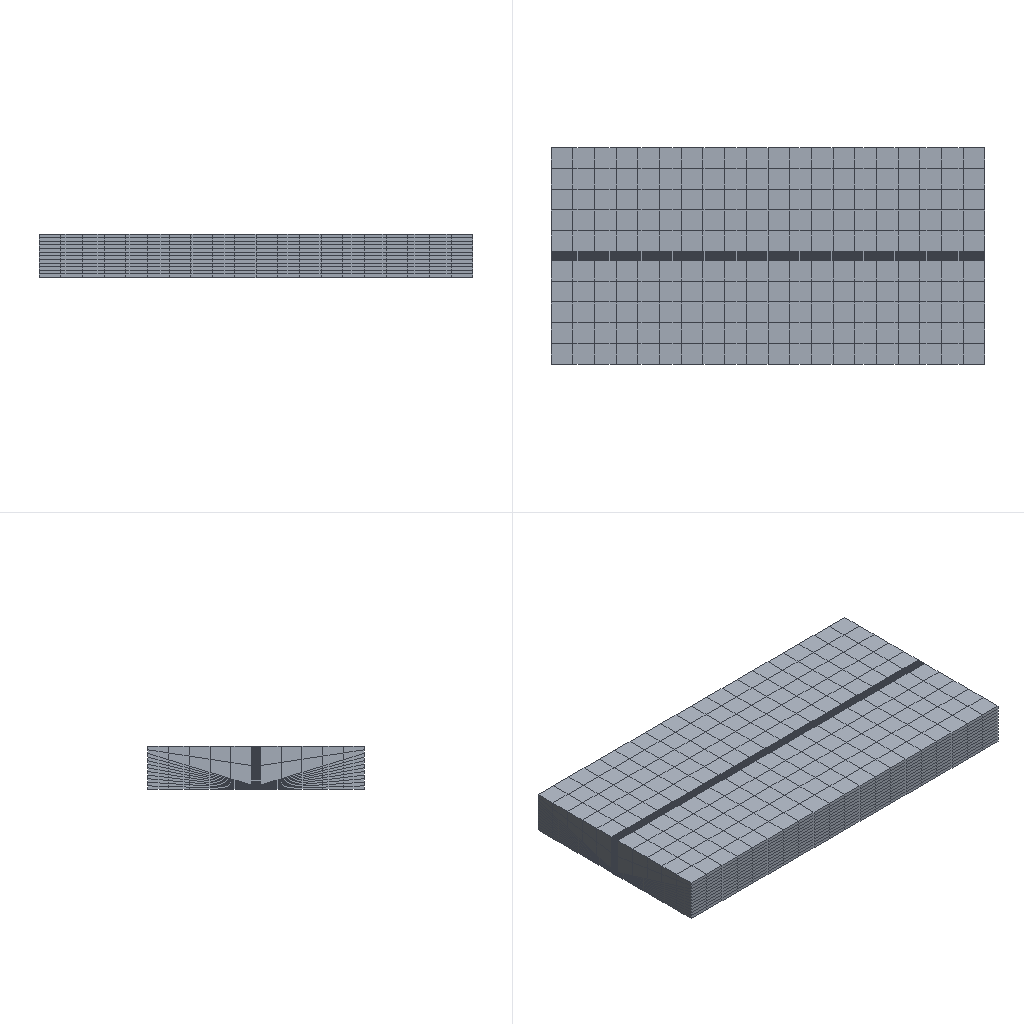Simulation study | abaqus
Set-up summary:
category,name,step,type,value,unit,region
solver,abaqus
solver,version,,,Abaqus/Standard 3DEXPERIENCE R2017x
units,not stated in the deck,,not stated
analysis,deck,,coupled temperature-displacement,coupled temperature-displacement
load_step,Step-1,Step-1,coupled temperature-displacement
load_step,requested,,,1
mesh,nodes,,,10685
mesh,elements,,,8200
element_type,C3D8RT,,solid,8200
load,load commands in deck,,count,3
bc,support commands in deck,,count,1
material,NI-TI,,in results
material,STEEL,,in results
check,setup vs results,,match,"per instance, exact: element labels, types and connectivity; labels of the nodes the elements use; coordinates of those nodes at SINGLE_PRECISION in 1 of 2 instance(s)"
Abaqus input file, long lists of numbers shortened:
*Heading
** Job name: 1011 Model name: Model-1
** Generated by: Abaqus/CAE 2017
*Preprint, echo=NO, model=NO, history=NO, contact=NO
**
** PARTS
**
*Part, name=Part-1
*Node
      1,           0.,         -24.,           0.
      2,           0.,         -26.,           0.
** (8461 more lines like these left out)
*Element, type=C3D8RT
   1,  212, 1201, 2821,  783,    1,   21,  403,   76
   2, 1201, 1202, 2822, 2821,   21,   22,  404,  403
** (7198 more lines like these left out)
*Nset, nset=Set-1, generate
    1,  8463,     1
*Elset, elset=Set-1, generate
    1,  7200,     1
** Section: STEEL
*Solid Section, elset=Set-1, material=STEEL
,
*End Part
**
*Part, name=Part-2
*Node
      1,         100.,          -1.,  0.1
      2,          99.,          -1.,  0.1
** (2220 more lines like these left out)
*Element, type=C3D8RT
   1,  203,  204,  305,  304,    1,    2,  103,  102
   2,  204,  205,  306,  305,    2,    3,  104,  103
** (998 more lines like these left out)
*Nset, nset=Set-1, generate
    1,  2222,     1
*Elset, elset=Set-1, generate
    1,  1000,     1
** Section: NI-TI
*Solid Section, elset=Set-1, material=NI-TI
,
*End Part
**
**
** ASSEMBLY
**
*Assembly, name=Assembly
**
*Instance, name=Part-1-1, part=Part-1
*End Instance
**
*Instance, name=Part-2-1, part=Part-2
          0.,        -24.5,         -0.1
*End Instance
**
*Node
      1,           0.,         -25., -0.1
*Node
      2,           0.,         -25., -0.1
*Nset, nset=Set-1, instance=Part-1-1
    1,    2,    3,    4,    7,   10,   13,   14,   15,   16,   17,   18,   19,   20,   21,   22
   23,   24,   25,   26,   27,   28,   29,   30,   31,   32,   33,   34,   35,   36,   37,   38
** (57 more lines like these left out)
*Nset, nset=Set-1, instance=Part-2-1, generate
    1,  2222,     1
*Elset, elset=Set-1, instance=Part-1-1
    1,    2,    3,    4,    5,    6,    7,    8,    9,   10,   11,   12,   13,   14,   15,   16
   17,   18,   19,   20,   21,   41,   61,   81,  101,  121,  141,  161,  181,  241,  242,  243
** (52 more lines like these left out)
*Elset, elset=Set-1, instance=Part-2-1, generate
    1,  1000,     1
*Nset, nset=Set-2, instance=Part-2-1, generate
    1,  2222,     1
*Elset, elset=Set-2, instance=Part-2-1, generate
    1,  1000,     1
*Nset, nset=Set-3, instance=Part-1-1
    1,    2,    7,   10,   18,   20,   21,   22,   23,   24,   25,   26,   27,   28,   29,   30
   31,   32,   33,   34,   35,   36,   37,   38,   39,   98,   99,  100,  101,  102,  103,  104
** (33 more lines like these left out)
*Elset, elset=Set-3, instance=Part-1-1
    1,    2,    3,    4,    5,    6,    7,    8,    9,   10,   11,   12,   13,   14,   15,   16
   17,   18,   19,   20,  241,  242,  243,  244,  245,  246,  247,  248,  249,  250,  251,  252
** (30 more lines like these left out)
*Nset, nset=Set-4, instance=Part-1-1, generate
    1,  8463,     1
*Nset, nset=Set-4, instance=Part-2-1, generate
    1,  2222,     1
*Elset, elset=Set-4, instance=Part-1-1, generate
    1,  7200,     1
*Elset, elset=Set-4, instance=Part-2-1, generate
    1,  1000,     1
*Nset, nset=Set-5, instance=Part-1-1
    5,    6,   11,   12,   14,   16,   17,   19,   78,   79,   80,   81,   82,   83,   84,   85
   86,   87,   88,   89,   90,   91,   92,   93,   94,   95,   96,  156,  157,  158,  159,  160
** (39 more lines like these left out)
*Elset, elset=Set-5, instance=Part-1-1
  221,  222,  223,  224,  225,  226,  227,  228,  229,  230,  231,  232,  233,  234,  235,  236
  237,  238,  239,  240,  461,  462,  463,  464,  465,  466,  467,  468,  469,  470,  471,  472
** (36 more lines like these left out)
*Nset, nset=Set-6, instance=Part-1-1, generate
    1,  8463,     1
*Nset, nset=Set-6, instance=Part-2-1, generate
    1,  2222,     1
*Elset, elset=Set-6, instance=Part-1-1, generate
    1,  7200,     1
*Elset, elset=Set-6, instance=Part-2-1, generate
    1,  1000,     1
*Elset, elset=_Surf-1_S5, internal, instance=Part-1-1
 6056, 6057, 6058, 6059, 6060, 6116, 6117, 6118, 6119, 6120, 6176, 6177, 6178, 6179, 6180, 6236
 6237, 6238, 6239, 6240, 6296, 6297, 6298, 6299, 6300, 6356, 6357, 6358, 6359, 6360, 6416, 6417
** (5 more lines like these left out)
*Elset, elset=_Surf-1_S5, internal, instance=Part-2-1, generate
    1,  1000,     1
*Elset, elset=_Surf-1_S3, internal, instance=Part-1-1
    1,    2,    3,    4,    5,    6,    7,    8,    9,   10,   11,   12,   13,   14,   15,   16
   17,   18,   19,   20,  241,  242,  243,  244,  245,  246,  247,  248,  249,  250,  251,  252
** (23 more lines like these left out)
*Elset, elset=_Surf-1_S3, internal, instance=Part-2-1, generate
    1,  1000,     1
*Elset, elset=_Surf-1_S4, internal, instance=Part-1-1
 4812, 4824, 4836, 4848, 4860, 4872, 4884, 4896, 4908, 4920, 4932, 4944, 4956, 4968, 4980, 4992
 5004, 5016, 5028, 5040, 5052, 5064, 5076, 5088, 5100, 5112, 5124, 5136, 5148, 5160, 5172, 5184
** (20 more lines like these left out)
*Elset, elset=_Surf-1_S4, internal, instance=Part-2-1, generate
  100,  1000,   100
*Elset, elset=_Surf-1_S1, internal, instance=Part-2-1, generate
  901,  1000,     1
*Elset, elset=_Surf-1_S2, internal, instance=Part-2-1, generate
   1,  100,    1
*Surface, type=ELEMENT, name=Surf-1
_Surf-1_S5, S5
_Surf-1_S3, S3
_Surf-1_S4, S4
_Surf-1_S2, S2
_Surf-1_S1, S1
*Elset, elset=_Surf-2_S5, internal, instance=Part-1-1
 6056, 6057, 6058, 6059, 6060, 6116, 6117, 6118, 6119, 6120, 6176, 6177, 6178, 6179, 6180, 6236
 6237, 6238, 6239, 6240, 6296, 6297, 6298, 6299, 6300, 6356, 6357, 6358, 6359, 6360, 6416, 6417
** (5 more lines like these left out)
*Elset, elset=_Surf-2_S5, internal, instance=Part-2-1, generate
    1,  1000,     1
*Elset, elset=_Surf-2_S3, internal, instance=Part-1-1
    1,    2,    3,    4,    5,    6,    7,    8,    9,   10,   11,   12,   13,   14,   15,   16
   17,   18,   19,   20,  241,  242,  243,  244,  245,  246,  247,  248,  249,  250,  251,  252
** (23 more lines like these left out)
*Elset, elset=_Surf-2_S3, internal, instance=Part-2-1, generate
    1,  1000,     1
*Elset, elset=_Surf-2_S4, internal, instance=Part-1-1
 4812, 4824, 4836, 4848, 4860, 4872, 4884, 4896, 4908, 4920, 4932, 4944, 4956, 4968, 4980, 4992
 5004, 5016, 5028, 5040, 5052, 5064, 5076, 5088, 5100, 5112, 5124, 5136, 5148, 5160, 5172, 5184
** (20 more lines like these left out)
*Elset, elset=_Surf-2_S4, internal, instance=Part-2-1, generate
  100,  1000,   100
*Elset, elset=_Surf-2_S1, internal, instance=Part-2-1, generate
  901,  1000,     1
*Elset, elset=_Surf-2_S2, internal, instance=Part-2-1, generate
   1,  100,    1
*Surface, type=ELEMENT, name=Surf-2
_Surf-2_S5, S5
_Surf-2_S3, S3
_Surf-2_S4, S4
_Surf-2_S2, S2
_Surf-2_S1, S1
*Elset, elset=_Surf-3_S2, internal, instance=Part-1-1
    1,    2,    3,    4,    5,    6,    7,    8,    9,   10,   11,   12,   13,   14,   15,   16
   17,   18,   19,   20,   21,   22,   23,   24,   25,   26,   27,   28,   29,   30,   31,   32
** (21 more lines like these left out)
*Elset, elset=_Surf-3_S2, internal, instance=Part-2-1, generate
   1,  100,    1
*Elset, elset=_Surf-3_S5, internal, instance=Part-1-1
  221,  222,  223,  224,  225,  226,  227,  228,  229,  230,  231,  232,  233,  234,  235,  236
  237,  238,  239,  240,  461,  462,  463,  464,  465,  466,  467,  468,  469,  470,  471,  472
** (45 more lines like these left out)
*Elset, elset=_Surf-3_S5, internal, instance=Part-2-1, generate
    1,  1000,     1
*Elset, elset=_Surf-3_S1, internal, instance=Part-1-1
 4561, 4562, 4563, 4564, 4565, 4566, 4567, 4568, 4569, 4570, 4571, 4572, 4573, 4574, 4575, 4576
 4577, 4578, 4579, 4580, 4581, 4582, 4583, 4584, 4585, 4586, 4587, 4588, 4589, 4590, 4591, 4592
** (21 more lines like these left out)
*Elset, elset=_Surf-3_S1, internal, instance=Part-2-1, generate
  901,  1000,     1
*Elset, elset=_Surf-3_S6, internal, instance=Part-1-1, generate
 4801,  5989,    12
*Elset, elset=_Surf-3_S6, internal, instance=Part-2-1, generate
   1,  901,  100
*Elset, elset=_Surf-3_S3, internal, instance=Part-1-1
    1,    2,    3,    4,    5,    6,    7,    8,    9,   10,   11,   12,   13,   14,   15,   16
   17,   18,   19,   20,  241,  242,  243,  244,  245,  246,  247,  248,  249,  250,  251,  252
** (30 more lines like these left out)
*Elset, elset=_Surf-3_S3, internal, instance=Part-2-1, generate
    1,  1000,     1
*Elset, elset=_Surf-3_S4, internal, instance=Part-1-1
 4812, 4824, 4836, 4848, 4860, 4872, 4884, 4896, 4908, 4920, 4932, 4944, 4956, 4968, 4980, 4992
 5004, 5016, 5028, 5040, 5052, 5064, 5076, 5088, 5100, 5112, 5124, 5136, 5148, 5160, 5172, 5184
** (20 more lines like these left out)
*Elset, elset=_Surf-3_S4, internal, instance=Part-2-1, generate
  100,  1000,   100
*Surface, type=ELEMENT, name=Surf-3
_Surf-3_S2, S2
_Surf-3_S5, S5
_Surf-3_S6, S6
_Surf-3_S4, S4
_Surf-3_S1, S1
_Surf-3_S3, S3
*Elset, elset=_Surf-4_S2, internal, instance=Part-1-1
    1,    2,    3,    4,    5,    6,    7,    8,    9,   10,   11,   12,   13,   14,   15,   16
   17,   18,   19,   20,   21,   22,   23,   24,   25,   26,   27,   28,   29,   30,   31,   32
** (21 more lines like these left out)
*Elset, elset=_Surf-4_S2, internal, instance=Part-2-1, generate
   1,  100,    1
*Elset, elset=_Surf-4_S5, internal, instance=Part-1-1
  221,  222,  223,  224,  225,  226,  227,  228,  229,  230,  231,  232,  233,  234,  235,  236
  237,  238,  239,  240,  461,  462,  463,  464,  465,  466,  467,  468,  469,  470,  471,  472
** (45 more lines like these left out)
*Elset, elset=_Surf-4_S5, internal, instance=Part-2-1, generate
    1,  1000,     1
*Elset, elset=_Surf-4_S1, internal, instance=Part-1-1
 4561, 4562, 4563, 4564, 4565, 4566, 4567, 4568, 4569, 4570, 4571, 4572, 4573, 4574, 4575, 4576
 4577, 4578, 4579, 4580, 4581, 4582, 4583, 4584, 4585, 4586, 4587, 4588, 4589, 4590, 4591, 4592
** (21 more lines like these left out)
*Elset, elset=_Surf-4_S1, internal, instance=Part-2-1, generate
  901,  1000,     1
*Elset, elset=_Surf-4_S6, internal, instance=Part-1-1, generate
 4801,  5989,    12
*Elset, elset=_Surf-4_S6, internal, instance=Part-2-1, generate
   1,  901,  100
*Elset, elset=_Surf-4_S3, internal, instance=Part-1-1
    1,    2,    3,    4,    5,    6,    7,    8,    9,   10,   11,   12,   13,   14,   15,   16
   17,   18,   19,   20,  241,  242,  243,  244,  245,  246,  247,  248,  249,  250,  251,  252
** (30 more lines like these left out)
*Elset, elset=_Surf-4_S3, internal, instance=Part-2-1, generate
    1,  1000,     1
*Elset, elset=_Surf-4_S4, internal, instance=Part-1-1
 4812, 4824, 4836, 4848, 4860, 4872, 4884, 4896, 4908, 4920, 4932, 4944, 4956, 4968, 4980, 4992
 5004, 5016, 5028, 5040, 5052, 5064, 5076, 5088, 5100, 5112, 5124, 5136, 5148, 5160, 5172, 5184
** (20 more lines like these left out)
*Elset, elset=_Surf-4_S4, internal, instance=Part-2-1, generate
  100,  1000,   100
*Surface, type=ELEMENT, name=Surf-4
_Surf-4_S2, S2
_Surf-4_S5, S5
_Surf-4_S6, S6
_Surf-4_S4, S4
_Surf-4_S1, S1
_Surf-4_S3, S3
*Elset, elset=_shang_S3, internal, instance=Part-1-1
    1,    2,    3,    4,    5,    6,    7,    8,    9,   10,   11,   12,   13,   14,   15,   16
   17,   18,   19,   20,  241,  242,  243,  244,  245,  246,  247,  248,  249,  250,  251,  252
** (23 more lines like these left out)
*Surface, type=ELEMENT, name=shang
_shang_S3, S3
*Elset, elset=_xia_S3, internal, instance=Part-2-1, generate
    1,  1000,     1
*Surface, type=ELEMENT, name=xia
_xia_S3, S3
** Constraint: Constraint-1
*Tie, name=Constraint-1, adjust=yes
shang, xia
*End Assembly
**
** MATERIALS
**
*Material, name=NI-TI
*Conductivity
10.,
*Density
 6.45e-09,
*Elastic
28000., 0.3
*Plastic
70.,0.
*Specific Heat
 3.2e+08,
*Material, name=STEEL
*Conductivity
 16.3,
*Density
 7.93e-09,
*Elastic
199000., 0.28
*Plastic
200.,0.
*Specific Heat
 5e+08,
**
** PHYSICAL CONSTANTS
**
*Physical Constants, absolute zero=-273.13, stefan boltzmann=5.67e-08
**
** PREDEFINED FIELDS
**
** Name: Predefined Field-1   Type: Temperature
*Initial Conditions, type=TEMPERATURE
Set-6, 20.
** ----------------------------------------------------------------
**
** STEP: Step-1
**
*Step, name=Step-1, nlgeom=YES
*Coupled Temperature-displacement, creep=none, deltmx=500., stabilize=0.0002, allsdtol=0.05, continue=NO
0.01, 1., 1e-05, 1.
**
** BOUNDARY CONDITIONS
**
** Name: BC-1 Type: 对称/反对称/完全固定
*Boundary
Set-5, ENCASTRE
**
** LOADS
**
** Name: Load-1   Type: Body heat flux
*Dflux
Set-4, BFNU, 1.
**
** INTERACTIONS
**
** Interaction: Int-1
*Sfilm
Surf-3, F, 20., 10.
** Interaction: Int-2
*Sradiate
Surf-4, R, 20., 0.3
**
** OUTPUT REQUESTS
**
*Restart, write, frequency=0
**
** FIELD OUTPUT: F-Output-1
**
*Output, field, number interval=100
*Node Output
NT, RF, U, V
*Element Output, directions=YES
E, HBF, HFL, MISES, PE, PEEQ, S, TEMP
*Contact Output
CSTRESS,
**
** HISTORY OUTPUT: H-Output-1
**
*Output, history, variable=PRESELECT
*End Step
Results summary:
result,step,,completed,increments=100 time=1.0/1.0
result,analysis,,,"coupled temperature-displacement, steady state"
result,last_loadstep,,,1
result,primary field,,,"U, NT11"
result,reaction total,,FX,0.0,model units
result,reaction total,,FY,0.0,model units
result,reaction total,,FZ,0.0,model units